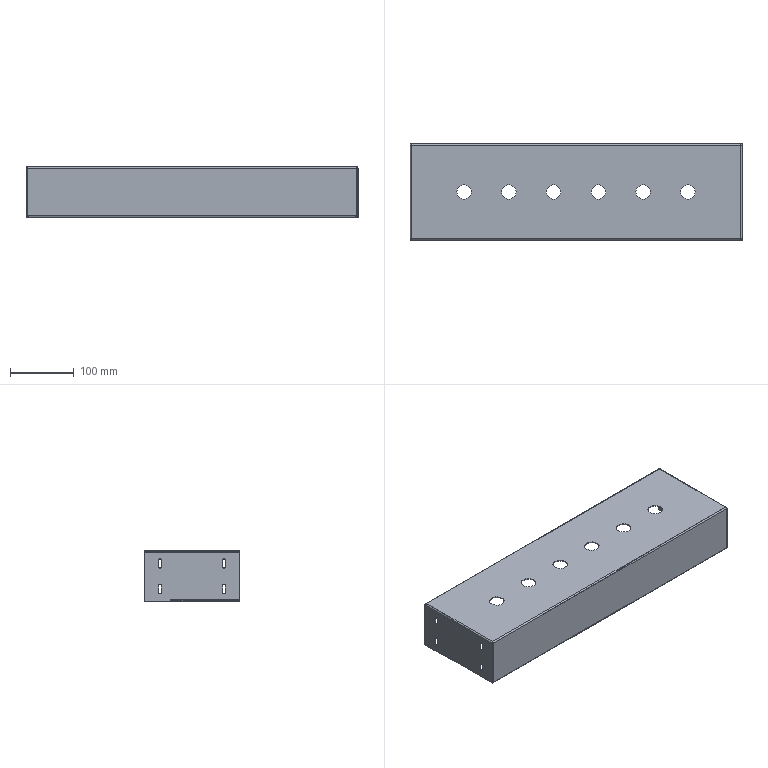Part | STEP file | 1 solid | 151 faces | box 519 x 150 x 79 mm | volume 247371 mm3 | plane 78 | cylinder 69 | spline 4 | commonest cylinder face diameters 4.5 x33 22.5 x12 1.2 x7 4.2 x7 3.3 x6 4 x4